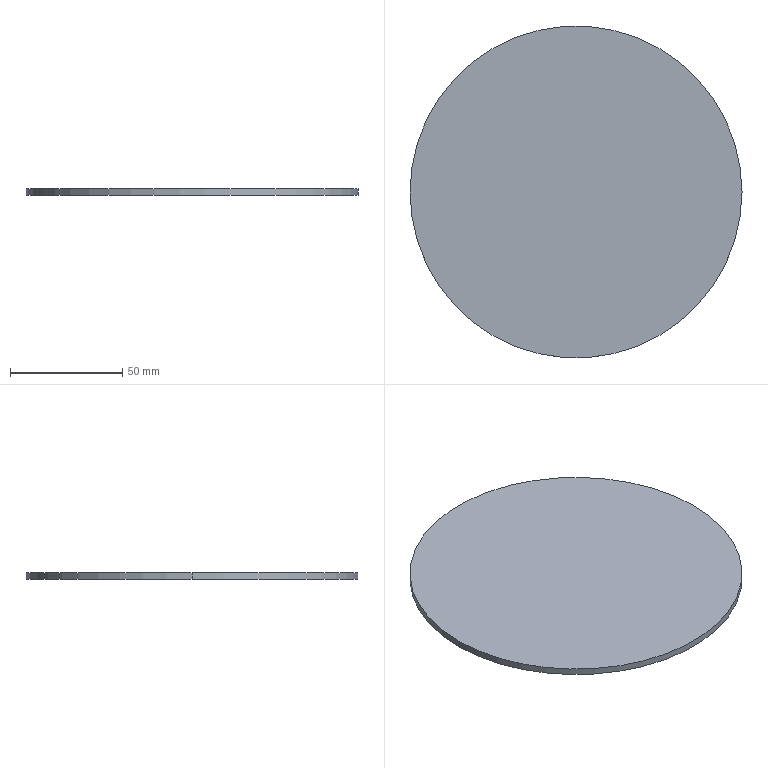Part | SolidWorks | features Extrusion 1 | 1 solid | 4 faces | box 148 x 148 x 3 mm | volume 51610 mm3 | cylinder 2 | plane 2 | commonest cylinder face diameters 148 x2
STEP:
#1=CARTESIAN_POINT('',(74.,0.,3.));
#2=VERTEX_POINT('',#1);
#3=CARTESIAN_POINT('',(-74.,0.,3.));
#4=VERTEX_POINT('',#3);
#5=CARTESIAN_POINT('',(0.,0.,3.));
#6=DIRECTION('',(0.,0.,1.));
#7=DIRECTION('',(1.,0.,0.));
#8=AXIS2_PLACEMENT_3D('',#5,#6,#7);
#9=CIRCLE('',#8,74.);
#10=EDGE_CURVE('',#2,#4,#9,.T.);
#11=ORIENTED_EDGE('',*,*,#10,.F.);
#12=CARTESIAN_POINT('',(74.,0.,0.));
#13=VERTEX_POINT('',#12);
#14=CARTESIAN_POINT('',(74.,0.,3.));
#15=DIRECTION('',(0.,0.,-1.));
#16=VECTOR('',#15,1000.);
#17=LINE('',#14,#16);
#18=EDGE_CURVE('',#2,#13,#17,.T.);
#19=ORIENTED_EDGE('',*,*,#18,.T.);
#20=CARTESIAN_POINT('',(-74.,0.,0.));
#21=VERTEX_POINT('',#20);
#22=CARTESIAN_POINT('',(0.,0.,0.));
#23=DIRECTION('',(0.,0.,1.));
#24=DIRECTION('',(1.,0.,0.));
#25=AXIS2_PLACEMENT_3D('',#22,#23,#24);
#26=CIRCLE('',#25,74.);
#27=EDGE_CURVE('',#13,#21,#26,.T.);
#28=ORIENTED_EDGE('',*,*,#27,.T.);
#29=CARTESIAN_POINT('',(-74.,0.,3.));
#30=DIRECTION('',(0.,0.,-1.));
#31=VECTOR('',#30,1000.);
#32=LINE('',#29,#31);
#33=EDGE_CURVE('',#4,#21,#32,.T.);
#34=ORIENTED_EDGE('',*,*,#33,.F.);
#35=EDGE_LOOP('',(#11,#19,#28,#34));
#36=FACE_OUTER_BOUND('',#35,.T.);
#37=CARTESIAN_POINT('',(0.,0.,3.));
#38=DIRECTION('',(0.,0.,-1.));
#39=DIRECTION('',(-1.,0.,0.));
#40=AXIS2_PLACEMENT_3D('',#37,#38,#39);
#41=CYLINDRICAL_SURFACE('',#40,74.);
#42=ADVANCED_FACE('',(#36),#41,.T.);
#43=ORIENTED_EDGE('',*,*,#18,.F.);
#44=CARTESIAN_POINT('',(0.,0.,3.));
#45=DIRECTION('',(0.,0.,1.));
#46=DIRECTION('',(1.,0.,0.));
#47=AXIS2_PLACEMENT_3D('',#44,#45,#46);
#48=CIRCLE('',#47,74.);
#49=EDGE_CURVE('',#4,#2,#48,.T.);
#50=ORIENTED_EDGE('',*,*,#49,.F.);
#51=ORIENTED_EDGE('',*,*,#33,.T.);
#52=CARTESIAN_POINT('',(0.,0.,0.));
#53=DIRECTION('',(0.,0.,1.));
#54=DIRECTION('',(1.,0.,0.));
#55=AXIS2_PLACEMENT_3D('',#52,#53,#54);
#56=CIRCLE('',#55,74.);
#57=EDGE_CURVE('',#21,#13,#56,.T.);
#58=ORIENTED_EDGE('',*,*,#57,.T.);
#59=EDGE_LOOP('',(#43,#50,#51,#58));
#60=FACE_OUTER_BOUND('',#59,.T.);
#61=CARTESIAN_POINT('',(0.,0.,3.));
#62=DIRECTION('',(0.,0.,-1.));
#63=DIRECTION('',(-1.,0.,0.));
#64=AXIS2_PLACEMENT_3D('',#61,#62,#63);
#65=CYLINDRICAL_SURFACE('',#64,74.);
#66=ADVANCED_FACE('',(#60),#65,.T.);
#67=ORIENTED_EDGE('',*,*,#49,.T.);
#68=ORIENTED_EDGE('',*,*,#10,.T.);
#69=EDGE_LOOP('',(#67,#68));
#70=FACE_OUTER_BOUND('',#69,.T.);
#71=CARTESIAN_POINT('',(0.,0.,3.));
#72=DIRECTION('',(0.,0.,1.));
#73=DIRECTION('',(1.,0.,0.));
#74=AXIS2_PLACEMENT_3D('',#71,#72,#73);
#75=PLANE('',#74);
#76=ADVANCED_FACE('',(#70),#75,.T.);
#77=ORIENTED_EDGE('',*,*,#57,.F.);
#78=ORIENTED_EDGE('',*,*,#27,.F.);
#79=EDGE_LOOP('',(#77,#78));
#80=FACE_OUTER_BOUND('',#79,.T.);
#81=CARTESIAN_POINT('',(0.,0.,0.));
#82=DIRECTION('',(0.,0.,1.));
#83=DIRECTION('',(1.,0.,0.));
#84=AXIS2_PLACEMENT_3D('',#81,#82,#83);
#85=PLANE('',#84);
#86=ADVANCED_FACE('',(#80),#85,.F.);
#87=CLOSED_SHELL('',(#42,#66,#76,#86));
#88=MANIFOLD_SOLID_BREP('',#87);
#89=CARTESIAN_POINT('',(0.,0.,0.));
#90=DIRECTION('',(0.,0.,1.));
#91=DIRECTION('',(1.,0.,0.));
#92=AXIS2_PLACEMENT_3D('',#89,#90,#91);
#93=(LENGTH_UNIT()NAMED_UNIT(*)SI_UNIT(.MILLI.,.METRE.));
#94=UNCERTAINTY_MEASURE_WITH_UNIT(LENGTH_MEASURE(0.00001),#93,'','');
#95=(NAMED_UNIT(*)PLANE_ANGLE_UNIT()SI_UNIT($,.RADIAN.));
#96=(NAMED_UNIT(*)SI_UNIT($,.STERADIAN.)SOLID_ANGLE_UNIT());
#97=(GEOMETRIC_REPRESENTATION_CONTEXT(3)GLOBAL_UNCERTAINTY_ASSIGNED_CONTEXT((#94))GLOBAL_UNIT_ASSIGNED_CONTEXT((#93,#95,#96))REPRESENTATION_CONTEXT('',''));
#98=ADVANCED_BREP_SHAPE_REPRESENTATION('',(#88,#92),#97);